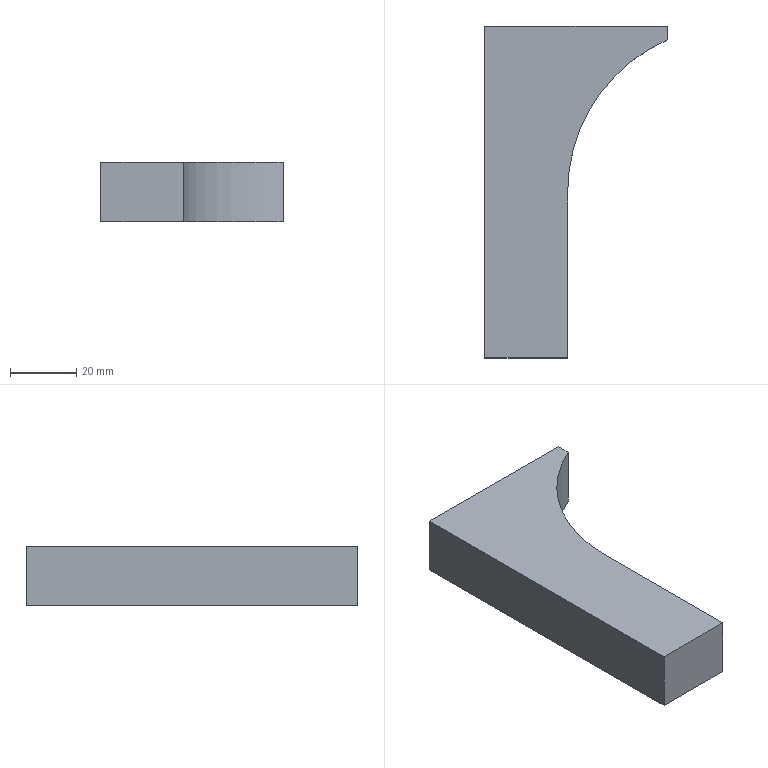Part | SolidWorks | features Extrusion 1 | 1 solid | 8 faces | box 55 x 100 x 18 mm | volume 54165 mm3 | plane 7 | cylinder 1 | commonest cylinder face diameters 100 x1
STEP:
#1=CARTESIAN_POINT('',(0.,0.,0.));
#2=VERTEX_POINT('',#1);
#3=CARTESIAN_POINT('',(25.,0.,0.));
#4=VERTEX_POINT('',#3);
#5=CARTESIAN_POINT('',(0.,0.,0.));
#6=DIRECTION('',(1.,0.,0.));
#7=VECTOR('',#6,1000.);
#8=LINE('',#5,#7);
#9=EDGE_CURVE('',#2,#4,#8,.T.);
#10=ORIENTED_EDGE('',*,*,#9,.T.);
#11=CARTESIAN_POINT('',(25.,0.,18.));
#12=VERTEX_POINT('',#11);
#13=CARTESIAN_POINT('',(25.,0.,18.));
#14=DIRECTION('',(0.,0.,-1.));
#15=VECTOR('',#14,1000.);
#16=LINE('',#13,#15);
#17=EDGE_CURVE('',#12,#4,#16,.T.);
#18=ORIENTED_EDGE('',*,*,#17,.F.);
#19=CARTESIAN_POINT('',(0.,0.,18.));
#20=VERTEX_POINT('',#19);
#21=CARTESIAN_POINT('',(0.,0.,18.));
#22=DIRECTION('',(1.,0.,0.));
#23=VECTOR('',#22,1000.);
#24=LINE('',#21,#23);
#25=EDGE_CURVE('',#20,#12,#24,.T.);
#26=ORIENTED_EDGE('',*,*,#25,.F.);
#27=CARTESIAN_POINT('',(0.,0.,18.));
#28=DIRECTION('',(0.,0.,-1.));
#29=VECTOR('',#28,1000.);
#30=LINE('',#27,#29);
#31=EDGE_CURVE('',#20,#2,#30,.T.);
#32=ORIENTED_EDGE('',*,*,#31,.T.);
#33=EDGE_LOOP('',(#10,#18,#26,#32));
#34=FACE_OUTER_BOUND('',#33,.T.);
#35=CARTESIAN_POINT('',(0.,0.,18.));
#36=DIRECTION('',(0.,1.,0.));
#37=DIRECTION('',(0.,0.,1.));
#38=AXIS2_PLACEMENT_3D('',#35,#36,#37);
#39=PLANE('',#38);
#40=ADVANCED_FACE('',(#34),#39,.F.);
#41=CARTESIAN_POINT('',(25.,50.,0.));
#42=VERTEX_POINT('',#41);
#43=CARTESIAN_POINT('',(25.,0.,0.));
#44=DIRECTION('',(0.,1.,0.));
#45=VECTOR('',#44,1000.);
#46=LINE('',#43,#45);
#47=EDGE_CURVE('',#4,#42,#46,.T.);
#48=ORIENTED_EDGE('',*,*,#47,.T.);
#49=CARTESIAN_POINT('',(25.,50.,18.));
#50=VERTEX_POINT('',#49);
#51=CARTESIAN_POINT('',(25.,50.,18.));
#52=DIRECTION('',(0.,0.,-1.));
#53=VECTOR('',#52,1000.);
#54=LINE('',#51,#53);
#55=EDGE_CURVE('',#50,#42,#54,.T.);
#56=ORIENTED_EDGE('',*,*,#55,.F.);
#57=CARTESIAN_POINT('',(25.,0.,18.));
#58=DIRECTION('',(0.,1.,0.));
#59=VECTOR('',#58,1000.);
#60=LINE('',#57,#59);
#61=EDGE_CURVE('',#12,#50,#60,.T.);
#62=ORIENTED_EDGE('',*,*,#61,.F.);
#63=ORIENTED_EDGE('',*,*,#17,.T.);
#64=EDGE_LOOP('',(#48,#56,#62,#63));
#65=FACE_OUTER_BOUND('',#64,.T.);
#66=CARTESIAN_POINT('',(25.,0.,18.));
#67=DIRECTION('',(-1.,0.,0.));
#68=DIRECTION('',(0.,0.,1.));
#69=AXIS2_PLACEMENT_3D('',#66,#67,#68);
#70=PLANE('',#69);
#71=ADVANCED_FACE('',(#65),#70,.F.);
#72=CARTESIAN_POINT('',(55.,95.826,0.));
#73=VERTEX_POINT('',#72);
#74=CARTESIAN_POINT('',(75.,50.,0.));
#75=DIRECTION('',(0.,0.,-1.));
#76=DIRECTION('',(1.,0.,0.));
#77=AXIS2_PLACEMENT_3D('',#74,#75,#76);
#78=CIRCLE('',#77,50.);
#79=EDGE_CURVE('',#42,#73,#78,.T.);
#80=ORIENTED_EDGE('',*,*,#79,.T.);
#81=CARTESIAN_POINT('',(55.,95.826,18.));
#82=VERTEX_POINT('',#81);
#83=CARTESIAN_POINT('',(55.,95.826,18.));
#84=DIRECTION('',(0.,0.,-1.));
#85=VECTOR('',#84,1000.);
#86=LINE('',#83,#85);
#87=EDGE_CURVE('',#82,#73,#86,.T.);
#88=ORIENTED_EDGE('',*,*,#87,.F.);
#89=CARTESIAN_POINT('',(75.,50.,18.));
#90=DIRECTION('',(0.,0.,-1.));
#91=DIRECTION('',(1.,0.,0.));
#92=AXIS2_PLACEMENT_3D('',#89,#90,#91);
#93=CIRCLE('',#92,50.);
#94=EDGE_CURVE('',#50,#82,#93,.T.);
#95=ORIENTED_EDGE('',*,*,#94,.F.);
#96=ORIENTED_EDGE('',*,*,#55,.T.);
#97=EDGE_LOOP('',(#80,#88,#95,#96));
#98=FACE_OUTER_BOUND('',#97,.T.);
#99=CARTESIAN_POINT('',(75.,50.,18.));
#100=DIRECTION('',(0.,0.,-1.));
#101=DIRECTION('',(-1.,0.,0.));
#102=AXIS2_PLACEMENT_3D('',#99,#100,#101);
#103=CYLINDRICAL_SURFACE('',#102,50.);
#104=ADVANCED_FACE('',(#98),#103,.F.);
#105=CARTESIAN_POINT('',(55.,100.,0.));
#106=VERTEX_POINT('',#105);
#107=CARTESIAN_POINT('',(55.,100.,0.));
#108=DIRECTION('',(0.,1.,0.));
#109=VECTOR('',#108,1000.);
#110=LINE('',#107,#109);
#111=EDGE_CURVE('',#73,#106,#110,.T.);
#112=ORIENTED_EDGE('',*,*,#111,.T.);
#113=CARTESIAN_POINT('',(55.,100.,18.));
#114=VERTEX_POINT('',#113);
#115=CARTESIAN_POINT('',(55.,100.,18.));
#116=DIRECTION('',(0.,0.,-1.));
#117=VECTOR('',#116,1000.);
#118=LINE('',#115,#117);
#119=EDGE_CURVE('',#114,#106,#118,.T.);
#120=ORIENTED_EDGE('',*,*,#119,.F.);
#121=CARTESIAN_POINT('',(55.,100.,18.));
#122=DIRECTION('',(0.,1.,0.));
#123=VECTOR('',#122,1000.);
#124=LINE('',#121,#123);
#125=EDGE_CURVE('',#82,#114,#124,.T.);
#126=ORIENTED_EDGE('',*,*,#125,.F.);
#127=ORIENTED_EDGE('',*,*,#87,.T.);
#128=EDGE_LOOP('',(#112,#120,#126,#127));
#129=FACE_OUTER_BOUND('',#128,.T.);
#130=CARTESIAN_POINT('',(55.,100.,18.));
#131=DIRECTION('',(-1.,0.,0.));
#132=DIRECTION('',(0.,0.,1.));
#133=AXIS2_PLACEMENT_3D('',#130,#131,#132);
#134=PLANE('',#133);
#135=ADVANCED_FACE('',(#129),#134,.F.);
#136=CARTESIAN_POINT('',(0.,100.,0.));
#137=VERTEX_POINT('',#136);
#138=CARTESIAN_POINT('',(0.,100.,0.));
#139=DIRECTION('',(-1.,0.,0.));
#140=VECTOR('',#139,1000.);
#141=LINE('',#138,#140);
#142=EDGE_CURVE('',#106,#137,#141,.T.);
#143=ORIENTED_EDGE('',*,*,#142,.T.);
#144=CARTESIAN_POINT('',(0.,100.,18.));
#145=VERTEX_POINT('',#144);
#146=CARTESIAN_POINT('',(0.,100.,18.));
#147=DIRECTION('',(0.,0.,-1.));
#148=VECTOR('',#147,1000.);
#149=LINE('',#146,#148);
#150=EDGE_CURVE('',#145,#137,#149,.T.);
#151=ORIENTED_EDGE('',*,*,#150,.F.);
#152=CARTESIAN_POINT('',(0.,100.,18.));
#153=DIRECTION('',(-1.,0.,0.));
#154=VECTOR('',#153,1000.);
#155=LINE('',#152,#154);
#156=EDGE_CURVE('',#114,#145,#155,.T.);
#157=ORIENTED_EDGE('',*,*,#156,.F.);
#158=ORIENTED_EDGE('',*,*,#119,.T.);
#159=EDGE_LOOP('',(#143,#151,#157,#158));
#160=FACE_OUTER_BOUND('',#159,.T.);
#161=CARTESIAN_POINT('',(0.,100.,18.));
#162=DIRECTION('',(0.,-1.,0.));
#163=DIRECTION('',(0.,0.,-1.));
#164=AXIS2_PLACEMENT_3D('',#161,#162,#163);
#165=PLANE('',#164);
#166=ADVANCED_FACE('',(#160),#165,.F.);
#167=CARTESIAN_POINT('',(0.,0.,0.));
#168=DIRECTION('',(0.,-1.,0.));
#169=VECTOR('',#168,1000.);
#170=LINE('',#167,#169);
#171=EDGE_CURVE('',#137,#2,#170,.T.);
#172=ORIENTED_EDGE('',*,*,#171,.T.);
#173=ORIENTED_EDGE('',*,*,#31,.F.);
#174=CARTESIAN_POINT('',(0.,0.,18.));
#175=DIRECTION('',(0.,-1.,0.));
#176=VECTOR('',#175,1000.);
#177=LINE('',#174,#176);
#178=EDGE_CURVE('',#145,#20,#177,.T.);
#179=ORIENTED_EDGE('',*,*,#178,.F.);
#180=ORIENTED_EDGE('',*,*,#150,.T.);
#181=EDGE_LOOP('',(#172,#173,#179,#180));
#182=FACE_OUTER_BOUND('',#181,.T.);
#183=CARTESIAN_POINT('',(0.,0.,18.));
#184=DIRECTION('',(1.,0.,0.));
#185=DIRECTION('',(0.,0.,-1.));
#186=AXIS2_PLACEMENT_3D('',#183,#184,#185);
#187=PLANE('',#186);
#188=ADVANCED_FACE('',(#182),#187,.F.);
#189=ORIENTED_EDGE('',*,*,#25,.T.);
#190=ORIENTED_EDGE('',*,*,#61,.T.);
#191=ORIENTED_EDGE('',*,*,#94,.T.);
#192=ORIENTED_EDGE('',*,*,#125,.T.);
#193=ORIENTED_EDGE('',*,*,#156,.T.);
#194=ORIENTED_EDGE('',*,*,#178,.T.);
#195=EDGE_LOOP('',(#189,#190,#191,#192,#193,#194));
#196=FACE_OUTER_BOUND('',#195,.T.);
#197=CARTESIAN_POINT('',(75.,50.,18.));
#198=DIRECTION('',(0.,0.,1.));
#199=DIRECTION('',(1.,0.,0.));
#200=AXIS2_PLACEMENT_3D('',#197,#198,#199);
#201=PLANE('',#200);
#202=ADVANCED_FACE('',(#196),#201,.T.);
#203=ORIENTED_EDGE('',*,*,#9,.F.);
#204=ORIENTED_EDGE('',*,*,#171,.F.);
#205=ORIENTED_EDGE('',*,*,#142,.F.);
#206=ORIENTED_EDGE('',*,*,#111,.F.);
#207=ORIENTED_EDGE('',*,*,#79,.F.);
#208=ORIENTED_EDGE('',*,*,#47,.F.);
#209=EDGE_LOOP('',(#203,#204,#205,#206,#207,#208));
#210=FACE_OUTER_BOUND('',#209,.T.);
#211=CARTESIAN_POINT('',(75.,50.,0.));
#212=DIRECTION('',(0.,0.,1.));
#213=DIRECTION('',(1.,0.,0.));
#214=AXIS2_PLACEMENT_3D('',#211,#212,#213);
#215=PLANE('',#214);
#216=ADVANCED_FACE('',(#210),#215,.F.);
#217=CLOSED_SHELL('',(#40,#71,#104,#135,#166,#188,#202,#216));
#218=MANIFOLD_SOLID_BREP('',#217);
#219=CARTESIAN_POINT('',(0.,0.,0.));
#220=DIRECTION('',(0.,0.,1.));
#221=DIRECTION('',(1.,0.,0.));
#222=AXIS2_PLACEMENT_3D('',#219,#220,#221);
#223=(LENGTH_UNIT()NAMED_UNIT(*)SI_UNIT(.MILLI.,.METRE.));
#224=UNCERTAINTY_MEASURE_WITH_UNIT(LENGTH_MEASURE(0.00001),#223,'','');
#225=(NAMED_UNIT(*)PLANE_ANGLE_UNIT()SI_UNIT($,.RADIAN.));
#226=(NAMED_UNIT(*)SI_UNIT($,.STERADIAN.)SOLID_ANGLE_UNIT());
#227=(GEOMETRIC_REPRESENTATION_CONTEXT(3)GLOBAL_UNCERTAINTY_ASSIGNED_CONTEXT((#224))GLOBAL_UNIT_ASSIGNED_CONTEXT((#223,#225,#226))REPRESENTATION_CONTEXT('',''));
#228=ADVANCED_BREP_SHAPE_REPRESENTATION('',(#218,#222),#227);